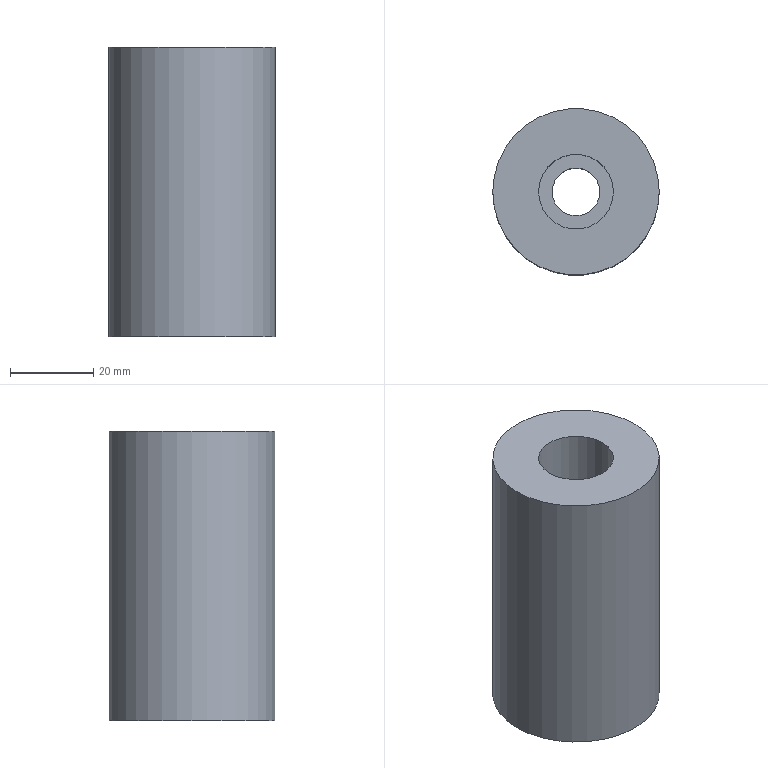Part | NX | features 27 2 | 1 solid | 6 faces | box 40 x 40 x 69.5 mm | volume 77181 mm3 | cylinder 3 | plane 3 | commonest cylinder face diameters 11.5 x1 18 x1 40 x1
STEP:
#1=CARTESIAN_POINT('',(2606.,0.,-113.));
#2=VERTEX_POINT('',#1);
#3=CARTESIAN_POINT('',(2626.,0.,-113.));
#4=DIRECTION('',(0.,0.,1.));
#5=DIRECTION('',(-1.,0.,0.));
#6=AXIS2_PLACEMENT_3D('',#3,#4,#5);
#7=CIRCLE('',#6,20.);
#8=EDGE_CURVE('',#2,#2,#7,.T.);
#9=ORIENTED_EDGE('',*,*,#8,.T.);
#10=EDGE_LOOP('',(#9));
#11=FACE_BOUND('',#10,.T.);
#12=CARTESIAN_POINT('',(2646.,0.,-43.5));
#13=VERTEX_POINT('',#12);
#14=CARTESIAN_POINT('',(2626.,0.,-43.5));
#15=DIRECTION('',(0.,0.,1.));
#16=DIRECTION('',(1.,0.,0.));
#17=AXIS2_PLACEMENT_3D('',#14,#15,#16);
#18=CIRCLE('',#17,20.);
#19=EDGE_CURVE('',#13,#13,#18,.T.);
#20=ORIENTED_EDGE('',*,*,#19,.F.);
#21=EDGE_LOOP('',(#20));
#22=FACE_BOUND('',#21,.T.);
#23=CARTESIAN_POINT('',(2626.,0.,30.));
#24=DIRECTION('',(0.,0.,1.));
#25=DIRECTION('',(-1.,0.,0.));
#26=AXIS2_PLACEMENT_3D('',#23,#24,#25);
#27=CYLINDRICAL_SURFACE('',#26,20.);
#28=ADVANCED_FACE('',(#11,#22),#27,.T.);
#29=CARTESIAN_POINT('',(2617.,0.,-63.));
#30=VERTEX_POINT('',#29);
#31=CARTESIAN_POINT('',(2626.,0.,-63.));
#32=DIRECTION('',(0.,0.,1.));
#33=DIRECTION('',(-1.,0.,0.));
#34=AXIS2_PLACEMENT_3D('',#31,#32,#33);
#35=CIRCLE('',#34,9.);
#36=EDGE_CURVE('',#30,#30,#35,.T.);
#37=ORIENTED_EDGE('',*,*,#36,.F.);
#38=EDGE_LOOP('',(#37));
#39=FACE_BOUND('',#38,.T.);
#40=CARTESIAN_POINT('',(2635.,0.,-43.5));
#41=VERTEX_POINT('',#40);
#42=CARTESIAN_POINT('',(2626.,0.,-43.5));
#43=DIRECTION('',(0.,0.,-1.));
#44=DIRECTION('',(1.,0.,0.));
#45=AXIS2_PLACEMENT_3D('',#42,#43,#44);
#46=CIRCLE('',#45,9.);
#47=EDGE_CURVE('',#41,#41,#46,.T.);
#48=ORIENTED_EDGE('',*,*,#47,.F.);
#49=EDGE_LOOP('',(#48));
#50=FACE_BOUND('',#49,.T.);
#51=CARTESIAN_POINT('',(2626.,0.,0.));
#52=DIRECTION('',(0.,0.,-1.));
#53=DIRECTION('',(-1.,0.,0.));
#54=AXIS2_PLACEMENT_3D('',#51,#52,#53);
#55=CYLINDRICAL_SURFACE('',#54,9.);
#56=ADVANCED_FACE('',(#39,#50),#55,.F.);
#57=CARTESIAN_POINT('',(2620.25,0.,-63.));
#58=VERTEX_POINT('',#57);
#59=CARTESIAN_POINT('',(2626.,0.,-63.));
#60=DIRECTION('',(0.,0.,1.));
#61=DIRECTION('',(-1.,0.,0.));
#62=AXIS2_PLACEMENT_3D('',#59,#60,#61);
#63=CIRCLE('',#62,5.75);
#64=EDGE_CURVE('',#58,#58,#63,.T.);
#65=ORIENTED_EDGE('',*,*,#64,.T.);
#66=EDGE_LOOP('',(#65));
#67=FACE_BOUND('',#66,.T.);
#68=CARTESIAN_POINT('',(2620.25,0.,-113.));
#69=VERTEX_POINT('',#68);
#70=CARTESIAN_POINT('',(2626.,0.,-113.));
#71=DIRECTION('',(0.,0.,1.));
#72=DIRECTION('',(-1.,0.,0.));
#73=AXIS2_PLACEMENT_3D('',#70,#71,#72);
#74=CIRCLE('',#73,5.75);
#75=EDGE_CURVE('',#69,#69,#74,.T.);
#76=ORIENTED_EDGE('',*,*,#75,.F.);
#77=EDGE_LOOP('',(#76));
#78=FACE_BOUND('',#77,.T.);
#79=CARTESIAN_POINT('',(2626.,0.,0.));
#80=DIRECTION('',(0.,0.,-1.));
#81=DIRECTION('',(-1.,0.,0.));
#82=AXIS2_PLACEMENT_3D('',#79,#80,#81);
#83=CYLINDRICAL_SURFACE('',#82,5.75);
#84=ADVANCED_FACE('',(#67,#78),#83,.F.);
#85=ORIENTED_EDGE('',*,*,#8,.F.);
#86=EDGE_LOOP('',(#85));
#87=FACE_BOUND('',#86,.T.);
#88=ORIENTED_EDGE('',*,*,#75,.T.);
#89=EDGE_LOOP('',(#88));
#90=FACE_BOUND('',#89,.T.);
#91=CARTESIAN_POINT('',(3198.5,260.,-113.));
#92=DIRECTION('',(0.,0.,-1.));
#93=DIRECTION('',(1.,0.,0.));
#94=AXIS2_PLACEMENT_3D('',#91,#92,#93);
#95=PLANE('',#94);
#96=ADVANCED_FACE('',(#87,#90),#95,.T.);
#97=ORIENTED_EDGE('',*,*,#64,.F.);
#98=EDGE_LOOP('',(#97));
#99=FACE_BOUND('',#98,.T.);
#100=ORIENTED_EDGE('',*,*,#36,.T.);
#101=EDGE_LOOP('',(#100));
#102=FACE_BOUND('',#101,.T.);
#103=CARTESIAN_POINT('',(2626.,0.,-63.));
#104=DIRECTION('',(0.,0.,-1.));
#105=DIRECTION('',(1.,0.,0.));
#106=AXIS2_PLACEMENT_3D('',#103,#104,#105);
#107=PLANE('',#106);
#108=ADVANCED_FACE('',(#99,#102),#107,.F.);
#109=ORIENTED_EDGE('',*,*,#47,.T.);
#110=EDGE_LOOP('',(#109));
#111=FACE_BOUND('',#110,.T.);
#112=ORIENTED_EDGE('',*,*,#19,.T.);
#113=EDGE_LOOP('',(#112));
#114=FACE_BOUND('',#113,.T.);
#115=CARTESIAN_POINT('',(2322.879,0.,-43.5));
#116=DIRECTION('',(0.,0.,1.));
#117=DIRECTION('',(-1.,0.,0.));
#118=AXIS2_PLACEMENT_3D('',#115,#116,#117);
#119=PLANE('',#118);
#120=ADVANCED_FACE('',(#111,#114),#119,.T.);
#121=CLOSED_SHELL('',(#28,#56,#84,#96,#108,#120));
#122=MANIFOLD_SOLID_BREP('',#121);
#123=(LENGTH_UNIT()NAMED_UNIT(*)SI_UNIT(.MILLI.,.METRE.));
#124=UNCERTAINTY_MEASURE_WITH_UNIT(LENGTH_MEASURE(0.00001),#123,'','');
#125=(NAMED_UNIT(*)PLANE_ANGLE_UNIT()SI_UNIT($,.RADIAN.));
#126=(NAMED_UNIT(*)SI_UNIT($,.STERADIAN.)SOLID_ANGLE_UNIT());
#127=(GEOMETRIC_REPRESENTATION_CONTEXT(3)GLOBAL_UNCERTAINTY_ASSIGNED_CONTEXT((#124))GLOBAL_UNIT_ASSIGNED_CONTEXT((#123,#125,#126))REPRESENTATION_CONTEXT('',''));
#128=ADVANCED_BREP_SHAPE_REPRESENTATION('',(#122),#127);